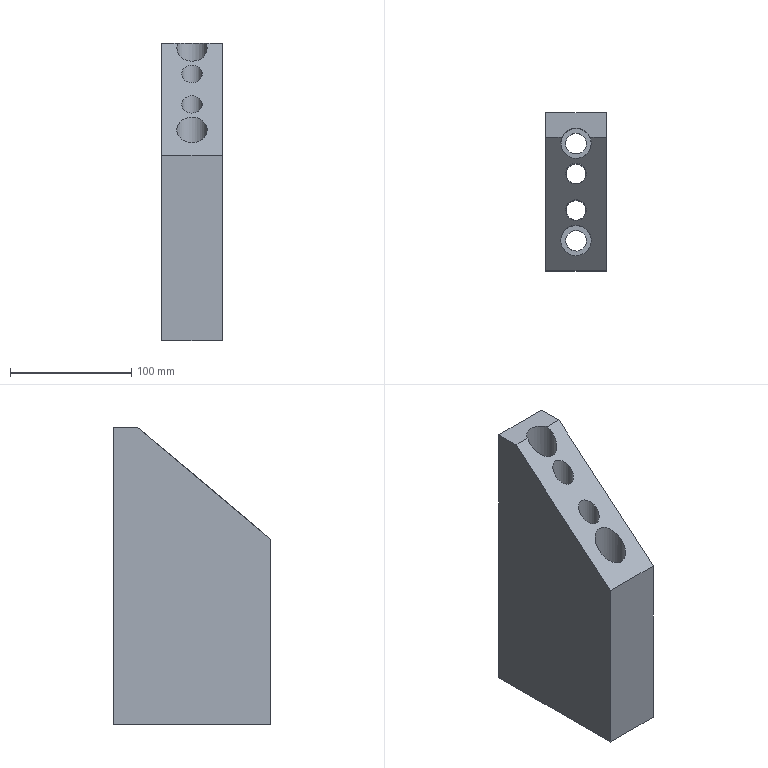Part | NX | features solid 2 | 1 solid | 19 faces | box 50 x 130 x 245 mm | volume 1058846 mm3 | plane 11 | cylinder 8 | commonest cylinder face diameters 17 x4 16 x2 25 x2
STEP:
#1=CARTESIAN_POINT('',(422.5,-300.,65.));
#2=VERTEX_POINT('',#1);
#3=CARTESIAN_POINT('',(422.5,-320.,65.));
#4=VERTEX_POINT('',#3);
#5=CARTESIAN_POINT('',(422.5,-300.,65.));
#6=DIRECTION('',(0.,-1.,0.));
#7=VECTOR('',#6,1000.);
#8=LINE('',#5,#7);
#9=EDGE_CURVE('',#2,#4,#8,.T.);
#10=ORIENTED_EDGE('',*,*,#9,.T.);
#11=CARTESIAN_POINT('',(422.5,-430.,-27.301));
#12=VERTEX_POINT('',#11);
#13=CARTESIAN_POINT('',(422.5,-390.902,5.507));
#14=DIRECTION('',(0.,-0.766,-0.6428));
#15=VECTOR('',#14,1000.);
#16=LINE('',#13,#15);
#17=EDGE_CURVE('',#4,#12,#16,.T.);
#18=ORIENTED_EDGE('',*,*,#17,.T.);
#19=CARTESIAN_POINT('',(422.5,-430.,-180.));
#20=VERTEX_POINT('',#19);
#21=CARTESIAN_POINT('',(422.5,-430.,25.));
#22=DIRECTION('',(0.,0.,-1.));
#23=VECTOR('',#22,1000.);
#24=LINE('',#21,#23);
#25=EDGE_CURVE('',#12,#20,#24,.T.);
#26=ORIENTED_EDGE('',*,*,#25,.T.);
#27=CARTESIAN_POINT('',(422.5,-300.,-180.));
#28=VERTEX_POINT('',#27);
#29=CARTESIAN_POINT('',(422.5,-300.,-180.));
#30=DIRECTION('',(0.,-1.,0.));
#31=VECTOR('',#30,1000.);
#32=LINE('',#29,#31);
#33=EDGE_CURVE('',#28,#20,#32,.T.);
#34=ORIENTED_EDGE('',*,*,#33,.F.);
#35=CARTESIAN_POINT('',(422.5,-300.,25.));
#36=DIRECTION('',(0.,0.,-1.));
#37=VECTOR('',#36,1000.);
#38=LINE('',#35,#37);
#39=EDGE_CURVE('',#2,#28,#38,.T.);
#40=ORIENTED_EDGE('',*,*,#39,.F.);
#41=EDGE_LOOP('',(#10,#18,#26,#34,#40));
#42=FACE_BOUND('',#41,.T.);
#43=CARTESIAN_POINT('',(422.5,-300.,25.));
#44=DIRECTION('',(-1.,0.,0.));
#45=DIRECTION('',(0.,0.,1.));
#46=AXIS2_PLACEMENT_3D('',#43,#44,#45);
#47=PLANE('',#46);
#48=ADVANCED_FACE('',(#42),#47,.F.);
#49=CARTESIAN_POINT('',(408.956,-320.,65.));
#50=VERTEX_POINT('',#49);
#51=CARTESIAN_POINT('',(386.044,-320.,65.));
#52=VERTEX_POINT('',#51);
#53=CARTESIAN_POINT('',(397.5,-325.,65.));
#54=DIRECTION('',(0.,0.,1.));
#55=DIRECTION('',(1.,0.,0.));
#56=AXIS2_PLACEMENT_3D('',#53,#54,#55);
#57=CIRCLE('',#56,12.5);
#58=EDGE_CURVE('',#50,#52,#57,.T.);
#59=ORIENTED_EDGE('',*,*,#58,.F.);
#60=CARTESIAN_POINT('',(447.5,-320.,65.));
#61=DIRECTION('',(1.,0.,0.));
#62=VECTOR('',#61,1000.);
#63=LINE('',#60,#62);
#64=EDGE_CURVE('',#50,#4,#63,.T.);
#65=ORIENTED_EDGE('',*,*,#64,.T.);
#66=ORIENTED_EDGE('',*,*,#9,.F.);
#67=CARTESIAN_POINT('',(372.5,-300.,65.));
#68=VERTEX_POINT('',#67);
#69=CARTESIAN_POINT('',(447.5,-300.,65.));
#70=DIRECTION('',(-1.,0.,0.));
#71=VECTOR('',#70,1000.);
#72=LINE('',#69,#71);
#73=EDGE_CURVE('',#2,#68,#72,.T.);
#74=ORIENTED_EDGE('',*,*,#73,.T.);
#75=CARTESIAN_POINT('',(372.5,-320.,65.));
#76=VERTEX_POINT('',#75);
#77=CARTESIAN_POINT('',(372.5,-300.,65.));
#78=DIRECTION('',(0.,-1.,0.));
#79=VECTOR('',#78,1000.);
#80=LINE('',#77,#79);
#81=EDGE_CURVE('',#68,#76,#80,.T.);
#82=ORIENTED_EDGE('',*,*,#81,.T.);
#83=CARTESIAN_POINT('',(447.5,-320.,65.));
#84=DIRECTION('',(1.,0.,0.));
#85=VECTOR('',#84,1000.);
#86=LINE('',#83,#85);
#87=EDGE_CURVE('',#76,#52,#86,.T.);
#88=ORIENTED_EDGE('',*,*,#87,.T.);
#89=EDGE_LOOP('',(#59,#65,#66,#74,#82,#88));
#90=FACE_BOUND('',#89,.T.);
#91=CARTESIAN_POINT('',(447.5,-300.,65.));
#92=DIRECTION('',(0.,0.,1.));
#93=DIRECTION('',(1.,0.,0.));
#94=AXIS2_PLACEMENT_3D('',#91,#92,#93);
#95=PLANE('',#94);
#96=ADVANCED_FACE('',(#90),#95,.T.);
#97=CARTESIAN_POINT('',(372.5,-430.,-180.));
#98=VERTEX_POINT('',#97);
#99=CARTESIAN_POINT('',(372.5,-430.,-27.301));
#100=VERTEX_POINT('',#99);
#101=CARTESIAN_POINT('',(372.5,-430.,-75.));
#102=DIRECTION('',(0.,0.,1.));
#103=VECTOR('',#102,1000.);
#104=LINE('',#101,#103);
#105=EDGE_CURVE('',#98,#100,#104,.T.);
#106=ORIENTED_EDGE('',*,*,#105,.T.);
#107=CARTESIAN_POINT('',(372.5,-390.902,5.507));
#108=DIRECTION('',(0.,0.766,0.6428));
#109=VECTOR('',#108,1000.);
#110=LINE('',#107,#109);
#111=EDGE_CURVE('',#100,#76,#110,.T.);
#112=ORIENTED_EDGE('',*,*,#111,.T.);
#113=ORIENTED_EDGE('',*,*,#81,.F.);
#114=CARTESIAN_POINT('',(372.5,-300.,-180.));
#115=VERTEX_POINT('',#114);
#116=CARTESIAN_POINT('',(372.5,-300.,-75.));
#117=DIRECTION('',(0.,0.,1.));
#118=VECTOR('',#117,1000.);
#119=LINE('',#116,#118);
#120=EDGE_CURVE('',#115,#68,#119,.T.);
#121=ORIENTED_EDGE('',*,*,#120,.F.);
#122=CARTESIAN_POINT('',(372.5,-300.,-180.));
#123=DIRECTION('',(0.,-1.,0.));
#124=VECTOR('',#123,1000.);
#125=LINE('',#122,#124);
#126=EDGE_CURVE('',#115,#98,#125,.T.);
#127=ORIENTED_EDGE('',*,*,#126,.T.);
#128=EDGE_LOOP('',(#106,#112,#113,#121,#127));
#129=FACE_BOUND('',#128,.T.);
#130=CARTESIAN_POINT('',(372.5,-300.,-75.));
#131=DIRECTION('',(1.,0.,0.));
#132=DIRECTION('',(0.,0.,-1.));
#133=AXIS2_PLACEMENT_3D('',#130,#131,#132);
#134=PLANE('',#133);
#135=ADVANCED_FACE('',(#129),#134,.F.);
#136=CARTESIAN_POINT('',(405.5,-380.,-180.));
#137=VERTEX_POINT('',#136);
#138=CARTESIAN_POINT('',(397.5,-380.,-180.));
#139=DIRECTION('',(0.,0.,1.));
#140=DIRECTION('',(1.,0.,0.));
#141=AXIS2_PLACEMENT_3D('',#138,#139,#140);
#142=CIRCLE('',#141,8.);
#143=EDGE_CURVE('',#137,#137,#142,.T.);
#144=ORIENTED_EDGE('',*,*,#143,.T.);
#145=EDGE_LOOP('',(#144));
#146=FACE_BOUND('',#145,.T.);
#147=CARTESIAN_POINT('',(405.5,-350.,-180.));
#148=VERTEX_POINT('',#147);
#149=CARTESIAN_POINT('',(397.5,-350.,-180.));
#150=DIRECTION('',(0.,0.,1.));
#151=DIRECTION('',(1.,0.,0.));
#152=AXIS2_PLACEMENT_3D('',#149,#150,#151);
#153=CIRCLE('',#152,8.);
#154=EDGE_CURVE('',#148,#148,#153,.T.);
#155=ORIENTED_EDGE('',*,*,#154,.T.);
#156=EDGE_LOOP('',(#155));
#157=FACE_BOUND('',#156,.T.);
#158=CARTESIAN_POINT('',(406.,-405.,-180.));
#159=VERTEX_POINT('',#158);
#160=CARTESIAN_POINT('',(397.5,-405.,-180.));
#161=DIRECTION('',(0.,0.,1.));
#162=DIRECTION('',(1.,0.,0.));
#163=AXIS2_PLACEMENT_3D('',#160,#161,#162);
#164=CIRCLE('',#163,8.5);
#165=EDGE_CURVE('',#159,#159,#164,.T.);
#166=ORIENTED_EDGE('',*,*,#165,.T.);
#167=EDGE_LOOP('',(#166));
#168=FACE_BOUND('',#167,.T.);
#169=CARTESIAN_POINT('',(406.,-325.,-180.));
#170=VERTEX_POINT('',#169);
#171=CARTESIAN_POINT('',(397.5,-325.,-180.));
#172=DIRECTION('',(0.,0.,1.));
#173=DIRECTION('',(1.,0.,0.));
#174=AXIS2_PLACEMENT_3D('',#171,#172,#173);
#175=CIRCLE('',#174,8.5);
#176=EDGE_CURVE('',#170,#170,#175,.T.);
#177=ORIENTED_EDGE('',*,*,#176,.T.);
#178=EDGE_LOOP('',(#177));
#179=FACE_BOUND('',#178,.T.);
#180=CARTESIAN_POINT('',(447.5,-430.,-180.));
#181=DIRECTION('',(-1.,0.,0.));
#182=VECTOR('',#181,1000.);
#183=LINE('',#180,#182);
#184=EDGE_CURVE('',#20,#98,#183,.T.);
#185=ORIENTED_EDGE('',*,*,#184,.T.);
#186=ORIENTED_EDGE('',*,*,#126,.F.);
#187=CARTESIAN_POINT('',(447.5,-300.,-180.));
#188=DIRECTION('',(-1.,0.,0.));
#189=VECTOR('',#188,1000.);
#190=LINE('',#187,#189);
#191=EDGE_CURVE('',#28,#115,#190,.T.);
#192=ORIENTED_EDGE('',*,*,#191,.F.);
#193=ORIENTED_EDGE('',*,*,#33,.T.);
#194=EDGE_LOOP('',(#185,#186,#192,#193));
#195=FACE_BOUND('',#194,.T.);
#196=CARTESIAN_POINT('',(447.5,-300.,-180.));
#197=DIRECTION('',(0.,0.,1.));
#198=DIRECTION('',(1.,0.,0.));
#199=AXIS2_PLACEMENT_3D('',#196,#197,#198);
#200=PLANE('',#199);
#201=ADVANCED_FACE('',(#146,#157,#168,#179,#195),#200,.F.);
#202=ORIENTED_EDGE('',*,*,#39,.T.);
#203=ORIENTED_EDGE('',*,*,#191,.T.);
#204=ORIENTED_EDGE('',*,*,#120,.T.);
#205=ORIENTED_EDGE('',*,*,#73,.F.);
#206=EDGE_LOOP('',(#202,#203,#204,#205));
#207=FACE_BOUND('',#206,.T.);
#208=CARTESIAN_POINT('',(447.5,-300.,25.));
#209=DIRECTION('',(0.,1.,0.));
#210=DIRECTION('',(-1.,0.,0.));
#211=AXIS2_PLACEMENT_3D('',#208,#209,#210);
#212=PLANE('',#211);
#213=ADVANCED_FACE('',(#207),#212,.T.);
#214=ORIENTED_EDGE('',*,*,#25,.F.);
#215=CARTESIAN_POINT('',(-205.,-430.,-27.301));
#216=DIRECTION('',(-1.,0.,0.));
#217=VECTOR('',#216,1000.);
#218=LINE('',#215,#217);
#219=EDGE_CURVE('',#12,#100,#218,.T.);
#220=ORIENTED_EDGE('',*,*,#219,.T.);
#221=ORIENTED_EDGE('',*,*,#105,.F.);
#222=ORIENTED_EDGE('',*,*,#184,.F.);
#223=EDGE_LOOP('',(#214,#220,#221,#222));
#224=FACE_BOUND('',#223,.T.);
#225=CARTESIAN_POINT('',(-205.,-430.,-120.405));
#226=DIRECTION('',(0.,1.,0.));
#227=DIRECTION('',(0.,0.,1.));
#228=AXIS2_PLACEMENT_3D('',#225,#226,#227);
#229=PLANE('',#228);
#230=ADVANCED_FACE('',(#224),#229,.F.);
#231=CARTESIAN_POINT('',(397.5,-371.5,21.786));
#232=VERTEX_POINT('',#231);
#233=CARTESIAN_POINT('',(397.5,-380.,14.654));
#234=DIRECTION('',(0.,-0.6428,0.766));
#235=DIRECTION('',(0.,0.766,0.6428));
#236=AXIS2_PLACEMENT_3D('',#233,#234,#235);
#237=ELLIPSE('',#236,11.096,8.5);
#238=EDGE_CURVE('',#232,#232,#237,.T.);
#239=ORIENTED_EDGE('',*,*,#238,.F.);
#240=EDGE_LOOP('',(#239));
#241=FACE_BOUND('',#240,.T.);
#242=CARTESIAN_POINT('',(397.5,-341.5,46.959));
#243=VERTEX_POINT('',#242);
#244=CARTESIAN_POINT('',(397.5,-350.,39.827));
#245=DIRECTION('',(0.,-0.6428,0.766));
#246=DIRECTION('',(0.,0.766,0.6428));
#247=AXIS2_PLACEMENT_3D('',#244,#245,#246);
#248=ELLIPSE('',#247,11.096,8.5);
#249=EDGE_CURVE('',#243,#243,#248,.T.);
#250=ORIENTED_EDGE('',*,*,#249,.F.);
#251=EDGE_LOOP('',(#250));
#252=FACE_BOUND('',#251,.T.);
#253=CARTESIAN_POINT('',(397.5,-392.5,4.165));
#254=VERTEX_POINT('',#253);
#255=CARTESIAN_POINT('',(397.5,-405.,-6.323));
#256=DIRECTION('',(0.,-0.6428,0.766));
#257=DIRECTION('',(0.,0.766,0.6428));
#258=AXIS2_PLACEMENT_3D('',#255,#256,#257);
#259=ELLIPSE('',#258,16.318,12.5);
#260=EDGE_CURVE('',#254,#254,#259,.T.);
#261=ORIENTED_EDGE('',*,*,#260,.F.);
#262=EDGE_LOOP('',(#261));
#263=FACE_BOUND('',#262,.T.);
#264=CARTESIAN_POINT('',(397.5,-325.,60.805));
#265=DIRECTION('',(0.,-0.6428,0.766));
#266=DIRECTION('',(0.,0.766,0.6428));
#267=AXIS2_PLACEMENT_3D('',#264,#265,#266);
#268=ELLIPSE('',#267,16.318,12.5);
#269=EDGE_CURVE('',#52,#50,#268,.T.);
#270=ORIENTED_EDGE('',*,*,#269,.F.);
#271=ORIENTED_EDGE('',*,*,#87,.F.);
#272=ORIENTED_EDGE('',*,*,#111,.F.);
#273=ORIENTED_EDGE('',*,*,#219,.F.);
#274=ORIENTED_EDGE('',*,*,#17,.F.);
#275=ORIENTED_EDGE('',*,*,#64,.F.);
#276=EDGE_LOOP('',(#270,#271,#272,#273,#274,#275));
#277=FACE_BOUND('',#276,.T.);
#278=CARTESIAN_POINT('',(-205.,-390.902,5.507));
#279=DIRECTION('',(0.,-0.6428,0.766));
#280=DIRECTION('',(0.,-0.766,-0.6428));
#281=AXIS2_PLACEMENT_3D('',#278,#279,#280);
#282=PLANE('',#281);
#283=ADVANCED_FACE('',(#241,#252,#263,#277),#282,.T.);
#284=CARTESIAN_POINT('',(389.,-325.,-150.));
#285=VERTEX_POINT('',#284);
#286=CARTESIAN_POINT('',(397.5,-325.,-150.));
#287=DIRECTION('',(0.,0.,-1.));
#288=DIRECTION('',(-1.,0.,0.));
#289=AXIS2_PLACEMENT_3D('',#286,#287,#288);
#290=CIRCLE('',#289,8.5);
#291=EDGE_CURVE('',#285,#285,#290,.F.);
#292=ORIENTED_EDGE('',*,*,#291,.T.);
#293=EDGE_LOOP('',(#292));
#294=FACE_BOUND('',#293,.T.);
#295=ORIENTED_EDGE('',*,*,#176,.F.);
#296=EDGE_LOOP('',(#295));
#297=FACE_BOUND('',#296,.T.);
#298=CARTESIAN_POINT('',(397.5,-325.,-210.));
#299=DIRECTION('',(0.,0.,1.));
#300=DIRECTION('',(1.,0.,0.));
#301=AXIS2_PLACEMENT_3D('',#298,#299,#300);
#302=CYLINDRICAL_SURFACE('',#301,8.5);
#303=ADVANCED_FACE('',(#294,#297),#302,.F.);
#304=ORIENTED_EDGE('',*,*,#291,.F.);
#305=EDGE_LOOP('',(#304));
#306=FACE_BOUND('',#305,.T.);
#307=CARTESIAN_POINT('',(410.,-325.,-150.));
#308=VERTEX_POINT('',#307);
#309=CARTESIAN_POINT('',(397.5,-325.,-150.));
#310=DIRECTION('',(0.,0.,1.));
#311=DIRECTION('',(1.,0.,0.));
#312=AXIS2_PLACEMENT_3D('',#309,#310,#311);
#313=CIRCLE('',#312,12.5);
#314=EDGE_CURVE('',#308,#308,#313,.T.);
#315=ORIENTED_EDGE('',*,*,#314,.T.);
#316=EDGE_LOOP('',(#315));
#317=FACE_BOUND('',#316,.T.);
#318=CARTESIAN_POINT('',(397.5,-325.,-150.));
#319=DIRECTION('',(0.,0.,-1.));
#320=DIRECTION('',(-1.,0.,0.));
#321=AXIS2_PLACEMENT_3D('',#318,#319,#320);
#322=PLANE('',#321);
#323=ADVANCED_FACE('',(#306,#317),#322,.F.);
#324=ORIENTED_EDGE('',*,*,#58,.T.);
#325=ORIENTED_EDGE('',*,*,#269,.T.);
#326=EDGE_LOOP('',(#324,#325));
#327=FACE_BOUND('',#326,.T.);
#328=ORIENTED_EDGE('',*,*,#314,.F.);
#329=EDGE_LOOP('',(#328));
#330=FACE_BOUND('',#329,.T.);
#331=CARTESIAN_POINT('',(397.5,-325.,-150.));
#332=DIRECTION('',(0.,0.,1.));
#333=DIRECTION('',(1.,0.,0.));
#334=AXIS2_PLACEMENT_3D('',#331,#332,#333);
#335=CYLINDRICAL_SURFACE('',#334,12.5);
#336=ADVANCED_FACE('',(#327,#330),#335,.F.);
#337=CARTESIAN_POINT('',(397.5,-396.5,-150.));
#338=VERTEX_POINT('',#337);
#339=CARTESIAN_POINT('',(397.5,-405.,-150.));
#340=DIRECTION('',(0.,0.,-1.));
#341=DIRECTION('',(0.,1.,0.));
#342=AXIS2_PLACEMENT_3D('',#339,#340,#341);
#343=CIRCLE('',#342,8.5);
#344=EDGE_CURVE('',#338,#338,#343,.F.);
#345=ORIENTED_EDGE('',*,*,#344,.T.);
#346=EDGE_LOOP('',(#345));
#347=FACE_BOUND('',#346,.T.);
#348=ORIENTED_EDGE('',*,*,#165,.F.);
#349=EDGE_LOOP('',(#348));
#350=FACE_BOUND('',#349,.T.);
#351=CARTESIAN_POINT('',(397.5,-405.,-210.));
#352=DIRECTION('',(0.,0.,1.));
#353=DIRECTION('',(0.,-1.,0.));
#354=AXIS2_PLACEMENT_3D('',#351,#352,#353);
#355=CYLINDRICAL_SURFACE('',#354,8.5);
#356=ADVANCED_FACE('',(#347,#350),#355,.F.);
#357=ORIENTED_EDGE('',*,*,#344,.F.);
#358=EDGE_LOOP('',(#357));
#359=FACE_BOUND('',#358,.T.);
#360=CARTESIAN_POINT('',(397.5,-417.5,-150.));
#361=VERTEX_POINT('',#360);
#362=CARTESIAN_POINT('',(397.5,-405.,-150.));
#363=DIRECTION('',(0.,0.,1.));
#364=DIRECTION('',(0.,-1.,0.));
#365=AXIS2_PLACEMENT_3D('',#362,#363,#364);
#366=CIRCLE('',#365,12.5);
#367=EDGE_CURVE('',#361,#361,#366,.T.);
#368=ORIENTED_EDGE('',*,*,#367,.T.);
#369=EDGE_LOOP('',(#368));
#370=FACE_BOUND('',#369,.T.);
#371=CARTESIAN_POINT('',(397.5,-405.,-150.));
#372=DIRECTION('',(0.,0.,-1.));
#373=DIRECTION('',(0.,1.,0.));
#374=AXIS2_PLACEMENT_3D('',#371,#372,#373);
#375=PLANE('',#374);
#376=ADVANCED_FACE('',(#359,#370),#375,.F.);
#377=ORIENTED_EDGE('',*,*,#260,.T.);
#378=EDGE_LOOP('',(#377));
#379=FACE_BOUND('',#378,.T.);
#380=ORIENTED_EDGE('',*,*,#367,.F.);
#381=EDGE_LOOP('',(#380));
#382=FACE_BOUND('',#381,.T.);
#383=CARTESIAN_POINT('',(397.5,-405.,-150.));
#384=DIRECTION('',(0.,0.,1.));
#385=DIRECTION('',(0.,-1.,0.));
#386=AXIS2_PLACEMENT_3D('',#383,#384,#385);
#387=CYLINDRICAL_SURFACE('',#386,12.5);
#388=ADVANCED_FACE('',(#379,#382),#387,.F.);
#389=CARTESIAN_POINT('',(389.5,-350.,-150.));
#390=VERTEX_POINT('',#389);
#391=CARTESIAN_POINT('',(397.5,-350.,-150.));
#392=DIRECTION('',(0.,0.,-1.));
#393=DIRECTION('',(-1.,0.,0.));
#394=AXIS2_PLACEMENT_3D('',#391,#392,#393);
#395=CIRCLE('',#394,8.);
#396=EDGE_CURVE('',#390,#390,#395,.F.);
#397=ORIENTED_EDGE('',*,*,#396,.T.);
#398=EDGE_LOOP('',(#397));
#399=FACE_BOUND('',#398,.T.);
#400=ORIENTED_EDGE('',*,*,#154,.F.);
#401=EDGE_LOOP('',(#400));
#402=FACE_BOUND('',#401,.T.);
#403=CARTESIAN_POINT('',(397.5,-350.,-210.));
#404=DIRECTION('',(0.,0.,1.));
#405=DIRECTION('',(1.,0.,0.));
#406=AXIS2_PLACEMENT_3D('',#403,#404,#405);
#407=CYLINDRICAL_SURFACE('',#406,8.);
#408=ADVANCED_FACE('',(#399,#402),#407,.F.);
#409=ORIENTED_EDGE('',*,*,#396,.F.);
#410=EDGE_LOOP('',(#409));
#411=FACE_BOUND('',#410,.T.);
#412=CARTESIAN_POINT('',(406.,-350.,-150.));
#413=VERTEX_POINT('',#412);
#414=CARTESIAN_POINT('',(397.5,-350.,-150.));
#415=DIRECTION('',(0.,0.,1.));
#416=DIRECTION('',(1.,0.,0.));
#417=AXIS2_PLACEMENT_3D('',#414,#415,#416);
#418=CIRCLE('',#417,8.5);
#419=EDGE_CURVE('',#413,#413,#418,.T.);
#420=ORIENTED_EDGE('',*,*,#419,.T.);
#421=EDGE_LOOP('',(#420));
#422=FACE_BOUND('',#421,.T.);
#423=CARTESIAN_POINT('',(397.5,-350.,-150.));
#424=DIRECTION('',(0.,0.,-1.));
#425=DIRECTION('',(-1.,0.,0.));
#426=AXIS2_PLACEMENT_3D('',#423,#424,#425);
#427=PLANE('',#426);
#428=ADVANCED_FACE('',(#411,#422),#427,.F.);
#429=ORIENTED_EDGE('',*,*,#249,.T.);
#430=EDGE_LOOP('',(#429));
#431=FACE_BOUND('',#430,.T.);
#432=ORIENTED_EDGE('',*,*,#419,.F.);
#433=EDGE_LOOP('',(#432));
#434=FACE_BOUND('',#433,.T.);
#435=CARTESIAN_POINT('',(397.5,-350.,-150.));
#436=DIRECTION('',(0.,0.,1.));
#437=DIRECTION('',(1.,0.,0.));
#438=AXIS2_PLACEMENT_3D('',#435,#436,#437);
#439=CYLINDRICAL_SURFACE('',#438,8.5);
#440=ADVANCED_FACE('',(#431,#434),#439,.F.);
#441=CARTESIAN_POINT('',(389.5,-380.,-150.));
#442=VERTEX_POINT('',#441);
#443=CARTESIAN_POINT('',(397.5,-380.,-150.));
#444=DIRECTION('',(0.,0.,-1.));
#445=DIRECTION('',(-1.,0.,0.));
#446=AXIS2_PLACEMENT_3D('',#443,#444,#445);
#447=CIRCLE('',#446,8.);
#448=EDGE_CURVE('',#442,#442,#447,.F.);
#449=ORIENTED_EDGE('',*,*,#448,.T.);
#450=EDGE_LOOP('',(#449));
#451=FACE_BOUND('',#450,.T.);
#452=ORIENTED_EDGE('',*,*,#143,.F.);
#453=EDGE_LOOP('',(#452));
#454=FACE_BOUND('',#453,.T.);
#455=CARTESIAN_POINT('',(397.5,-380.,-210.));
#456=DIRECTION('',(0.,0.,1.));
#457=DIRECTION('',(1.,0.,0.));
#458=AXIS2_PLACEMENT_3D('',#455,#456,#457);
#459=CYLINDRICAL_SURFACE('',#458,8.);
#460=ADVANCED_FACE('',(#451,#454),#459,.F.);
#461=ORIENTED_EDGE('',*,*,#448,.F.);
#462=EDGE_LOOP('',(#461));
#463=FACE_BOUND('',#462,.T.);
#464=CARTESIAN_POINT('',(406.,-380.,-150.));
#465=VERTEX_POINT('',#464);
#466=CARTESIAN_POINT('',(397.5,-380.,-150.));
#467=DIRECTION('',(0.,0.,1.));
#468=DIRECTION('',(1.,0.,0.));
#469=AXIS2_PLACEMENT_3D('',#466,#467,#468);
#470=CIRCLE('',#469,8.5);
#471=EDGE_CURVE('',#465,#465,#470,.T.);
#472=ORIENTED_EDGE('',*,*,#471,.T.);
#473=EDGE_LOOP('',(#472));
#474=FACE_BOUND('',#473,.T.);
#475=CARTESIAN_POINT('',(397.5,-380.,-150.));
#476=DIRECTION('',(0.,0.,-1.));
#477=DIRECTION('',(-1.,0.,0.));
#478=AXIS2_PLACEMENT_3D('',#475,#476,#477);
#479=PLANE('',#478);
#480=ADVANCED_FACE('',(#463,#474),#479,.F.);
#481=ORIENTED_EDGE('',*,*,#238,.T.);
#482=EDGE_LOOP('',(#481));
#483=FACE_BOUND('',#482,.T.);
#484=ORIENTED_EDGE('',*,*,#471,.F.);
#485=EDGE_LOOP('',(#484));
#486=FACE_BOUND('',#485,.T.);
#487=CARTESIAN_POINT('',(397.5,-380.,-150.));
#488=DIRECTION('',(0.,0.,1.));
#489=DIRECTION('',(1.,0.,0.));
#490=AXIS2_PLACEMENT_3D('',#487,#488,#489);
#491=CYLINDRICAL_SURFACE('',#490,8.5);
#492=ADVANCED_FACE('',(#483,#486),#491,.F.);
#493=CLOSED_SHELL('',(#48,#96,#135,#201,#213,#230,#283,#303,#323,#336,#356,#376,#388,#408,#428,#440,#460,#480,#492));
#494=MANIFOLD_SOLID_BREP('',#493);
#495=(LENGTH_UNIT()NAMED_UNIT(*)SI_UNIT(.MILLI.,.METRE.));
#496=UNCERTAINTY_MEASURE_WITH_UNIT(LENGTH_MEASURE(0.00001),#495,'','');
#497=(NAMED_UNIT(*)PLANE_ANGLE_UNIT()SI_UNIT($,.RADIAN.));
#498=(NAMED_UNIT(*)SI_UNIT($,.STERADIAN.)SOLID_ANGLE_UNIT());
#499=(GEOMETRIC_REPRESENTATION_CONTEXT(3)GLOBAL_UNCERTAINTY_ASSIGNED_CONTEXT((#496))GLOBAL_UNIT_ASSIGNED_CONTEXT((#495,#497,#498))REPRESENTATION_CONTEXT('',''));
#500=ADVANCED_BREP_SHAPE_REPRESENTATION('',(#494),#499);